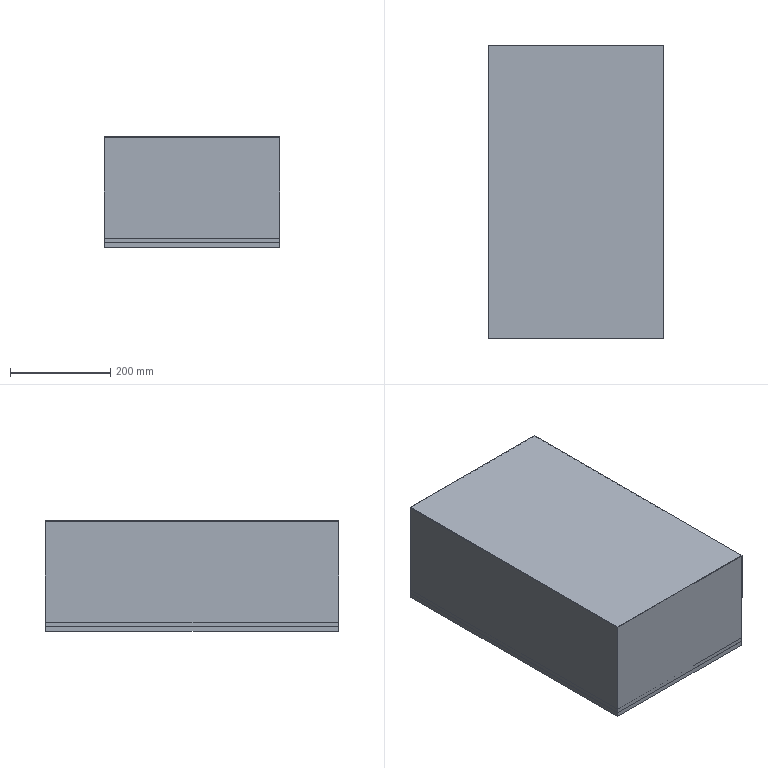Part | STEP file | Electrical box | 32 solids | 3845 faces | volume 11408010 mm3 | spline 3828 | plane 17